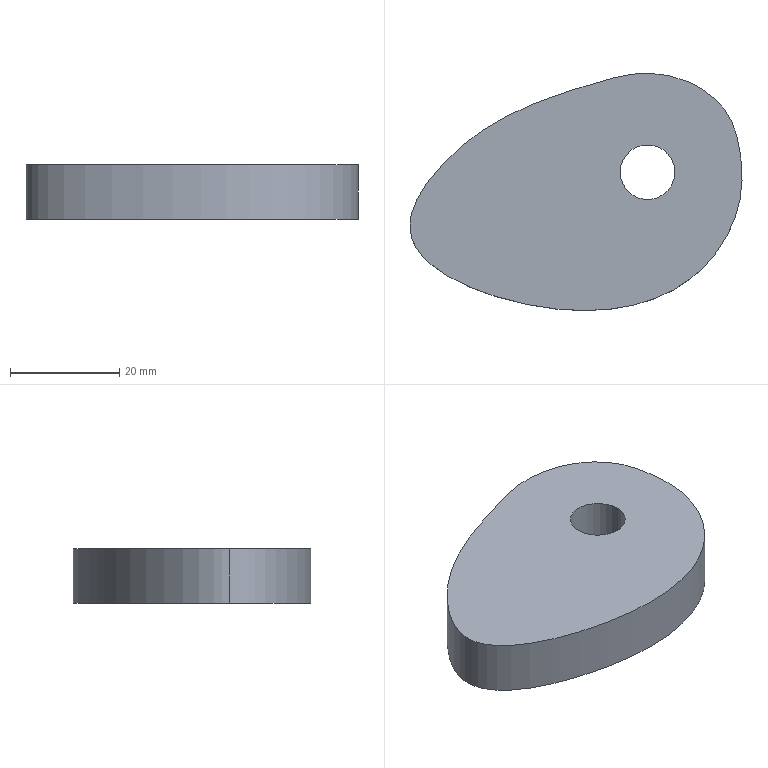Part | SolidWorks | features Extrusion 1 | 1 solid | 6 faces | box 60.725 x 43.378 x 10 mm | volume 18972 mm3 | cylinder 2 | spline 2 | plane 2 | commonest cylinder face diameters 10 x2
STEP:
#1=CARTESIAN_POINT('',(-5.,0.,10.));
#2=VERTEX_POINT('',#1);
#3=CARTESIAN_POINT('',(5.,0.,10.));
#4=VERTEX_POINT('',#3);
#5=CARTESIAN_POINT('',(0.,0.,10.));
#6=DIRECTION('',(0.,0.,1.));
#7=DIRECTION('',(1.,0.,0.));
#8=AXIS2_PLACEMENT_3D('',#5,#6,#7);
#9=CIRCLE('',#8,5.);
#10=EDGE_CURVE('',#2,#4,#9,.T.);
#11=ORIENTED_EDGE('',*,*,#10,.T.);
#12=CARTESIAN_POINT('',(5.,0.,0.));
#13=VERTEX_POINT('',#12);
#14=CARTESIAN_POINT('',(5.,0.,10.));
#15=DIRECTION('',(0.,0.,-1.));
#16=VECTOR('',#15,1000.);
#17=LINE('',#14,#16);
#18=EDGE_CURVE('',#4,#13,#17,.T.);
#19=ORIENTED_EDGE('',*,*,#18,.T.);
#20=CARTESIAN_POINT('',(-5.,0.,0.));
#21=VERTEX_POINT('',#20);
#22=CARTESIAN_POINT('',(0.,0.,0.));
#23=DIRECTION('',(0.,0.,1.));
#24=DIRECTION('',(1.,0.,0.));
#25=AXIS2_PLACEMENT_3D('',#22,#23,#24);
#26=CIRCLE('',#25,5.);
#27=EDGE_CURVE('',#21,#13,#26,.T.);
#28=ORIENTED_EDGE('',*,*,#27,.F.);
#29=CARTESIAN_POINT('',(-5.,0.,10.));
#30=DIRECTION('',(0.,0.,-1.));
#31=VECTOR('',#30,1000.);
#32=LINE('',#29,#31);
#33=EDGE_CURVE('',#2,#21,#32,.T.);
#34=ORIENTED_EDGE('',*,*,#33,.F.);
#35=EDGE_LOOP('',(#11,#19,#28,#34));
#36=FACE_OUTER_BOUND('',#35,.T.);
#37=CARTESIAN_POINT('',(0.,0.,10.));
#38=DIRECTION('',(0.,0.,-1.));
#39=DIRECTION('',(-1.,0.,0.));
#40=AXIS2_PLACEMENT_3D('',#37,#38,#39);
#41=CYLINDRICAL_SURFACE('',#40,5.);
#42=ADVANCED_FACE('',(#36),#41,.F.);
#43=CARTESIAN_POINT('',(-43.419,-10.499,10.));
#44=VERTEX_POINT('',#43);
#45=CARTESIAN_POINT('',(17.013,2.958,10.));
#46=VERTEX_POINT('',#45);
#47=CARTESIAN_POINT('',(-43.419,-10.499,10.));
#48=CARTESIAN_POINT('',(-42.752,-17.454,10.));
#49=CARTESIAN_POINT('',(-17.056,-28.779,10.));
#50=CARTESIAN_POINT('',(9.041,-23.635,10.));
#51=CARTESIAN_POINT('',(17.515,-6.091,10.));
#52=CARTESIAN_POINT('',(17.324,0.4877,10.));
#53=CARTESIAN_POINT('',(17.013,2.958,10.));
#54=B_SPLINE_CURVE_WITH_KNOTS('',3,(#47,#48,#49,#50,#51,#52,#53),.UNSPECIFIED.,.F.,.F.,(4,1,1,1,4),(0.5,0.6591,0.8767,0.9539,1.),.UNSPECIFIED.);
#55=EDGE_CURVE('',#44,#46,#54,.T.);
#56=ORIENTED_EDGE('',*,*,#55,.F.);
#57=CARTESIAN_POINT('',(-43.419,-10.499,0.));
#58=VERTEX_POINT('',#57);
#59=CARTESIAN_POINT('',(-43.419,-10.499,10.));
#60=DIRECTION('',(0.,0.,-1.));
#61=VECTOR('',#60,1000.);
#62=LINE('',#59,#61);
#63=EDGE_CURVE('',#44,#58,#62,.T.);
#64=ORIENTED_EDGE('',*,*,#63,.T.);
#65=CARTESIAN_POINT('',(17.013,2.958,0.));
#66=VERTEX_POINT('',#65);
#67=CARTESIAN_POINT('',(-43.419,-10.499,0.));
#68=CARTESIAN_POINT('',(-42.752,-17.454,0.));
#69=CARTESIAN_POINT('',(-17.056,-28.779,0.));
#70=CARTESIAN_POINT('',(9.041,-23.635,0.));
#71=CARTESIAN_POINT('',(17.515,-6.091,0.));
#72=CARTESIAN_POINT('',(17.324,0.4877,0.));
#73=CARTESIAN_POINT('',(17.013,2.958,0.));
#74=B_SPLINE_CURVE_WITH_KNOTS('',3,(#67,#68,#69,#70,#71,#72,#73),.UNSPECIFIED.,.F.,.F.,(4,1,1,1,4),(0.5,0.6591,0.8767,0.9539,1.),.UNSPECIFIED.);
#75=EDGE_CURVE('',#58,#66,#74,.T.);
#76=ORIENTED_EDGE('',*,*,#75,.T.);
#77=CARTESIAN_POINT('',(17.013,2.958,10.));
#78=DIRECTION('',(0.,0.,-1.));
#79=VECTOR('',#78,1000.);
#80=LINE('',#77,#79);
#81=EDGE_CURVE('',#46,#66,#80,.T.);
#82=ORIENTED_EDGE('',*,*,#81,.F.);
#83=EDGE_LOOP('',(#56,#64,#76,#82));
#84=FACE_OUTER_BOUND('',#83,.T.);
#85=CARTESIAN_POINT('',(-43.419,-10.499,10.));
#86=CARTESIAN_POINT('',(-43.419,-10.499,0.));
#87=CARTESIAN_POINT('',(-42.752,-17.454,10.));
#88=CARTESIAN_POINT('',(-42.752,-17.454,0.));
#89=CARTESIAN_POINT('',(-17.056,-28.779,10.));
#90=CARTESIAN_POINT('',(-17.056,-28.779,0.));
#91=CARTESIAN_POINT('',(9.041,-23.635,10.));
#92=CARTESIAN_POINT('',(9.041,-23.635,0.));
#93=CARTESIAN_POINT('',(17.515,-6.091,10.));
#94=CARTESIAN_POINT('',(17.515,-6.091,0.));
#95=CARTESIAN_POINT('',(17.324,0.4877,10.));
#96=CARTESIAN_POINT('',(17.324,0.4877,0.));
#97=CARTESIAN_POINT('',(17.013,2.958,10.));
#98=CARTESIAN_POINT('',(17.013,2.958,0.));
#99=B_SPLINE_SURFACE_WITH_KNOTS('',3,1,((#85,#86),(#87,#88),(#89,#90),(#91,#92),(#93,#94),(#95,#96),(#97,#98)),.UNSPECIFIED.,.F.,.F.,.F.,(4,1,1,1,4),(2,2),(0.5,0.6591,0.8767,0.9539,1.),(0.,1.),.UNSPECIFIED.);
#100=ADVANCED_FACE('',(#84),#99,.F.);
#101=CARTESIAN_POINT('',(17.013,2.958,10.));
#102=CARTESIAN_POINT('',(16.67,5.672,10.));
#103=CARTESIAN_POINT('',(15.377,11.266,10.));
#104=CARTESIAN_POINT('',(8.,17.178,10.));
#105=CARTESIAN_POINT('',(-1.479,18.809,10.));
#106=CARTESIAN_POINT('',(-16.415,14.213,10.));
#107=CARTESIAN_POINT('',(-32.42,9.014,10.));
#108=CARTESIAN_POINT('',(-43.748,-5.66,10.));
#109=CARTESIAN_POINT('',(-43.432,-10.363,10.));
#110=CARTESIAN_POINT('',(-43.419,-10.499,10.));
#111=B_SPLINE_CURVE_WITH_KNOTS('',3,(#101,#102,#103,#104,#105,#106,#107,#108,#109,#110),.UNSPECIFIED.,.F.,.F.,(4,1,1,1,1,1,1,4),(0.,0.05062,0.1037,0.1669,0.2236,0.393,0.4969,0.5),.UNSPECIFIED.);
#112=EDGE_CURVE('',#46,#44,#111,.T.);
#113=ORIENTED_EDGE('',*,*,#112,.T.);
#114=ORIENTED_EDGE('',*,*,#55,.T.);
#115=EDGE_LOOP('',(#113,#114));
#116=FACE_OUTER_BOUND('',#115,.T.);
#117=ORIENTED_EDGE('',*,*,#10,.F.);
#118=CARTESIAN_POINT('',(0.,0.,10.));
#119=DIRECTION('',(0.,0.,1.));
#120=DIRECTION('',(1.,0.,0.));
#121=AXIS2_PLACEMENT_3D('',#118,#119,#120);
#122=CIRCLE('',#121,5.);
#123=EDGE_CURVE('',#4,#2,#122,.T.);
#124=ORIENTED_EDGE('',*,*,#123,.F.);
#125=EDGE_LOOP('',(#117,#124));
#126=FACE_BOUND('',#125,.T.);
#127=CARTESIAN_POINT('',(-43.419,-10.499,10.));
#128=DIRECTION('',(0.,0.,-1.));
#129=DIRECTION('',(-1.,0.,0.));
#130=AXIS2_PLACEMENT_3D('',#127,#128,#129);
#131=PLANE('',#130);
#132=ADVANCED_FACE('',(#116,#126),#131,.F.);
#133=CARTESIAN_POINT('',(17.013,2.958,0.));
#134=CARTESIAN_POINT('',(16.67,5.672,0.));
#135=CARTESIAN_POINT('',(15.377,11.266,0.));
#136=CARTESIAN_POINT('',(8.,17.178,0.));
#137=CARTESIAN_POINT('',(-1.479,18.809,0.));
#138=CARTESIAN_POINT('',(-16.415,14.213,0.));
#139=CARTESIAN_POINT('',(-32.42,9.014,0.));
#140=CARTESIAN_POINT('',(-43.748,-5.66,0.));
#141=CARTESIAN_POINT('',(-43.432,-10.363,0.));
#142=CARTESIAN_POINT('',(-43.419,-10.499,0.));
#143=B_SPLINE_CURVE_WITH_KNOTS('',3,(#133,#134,#135,#136,#137,#138,#139,#140,#141,#142),.UNSPECIFIED.,.F.,.F.,(4,1,1,1,1,1,1,4),(0.,0.05062,0.1037,0.1669,0.2236,0.393,0.4969,0.5),.UNSPECIFIED.);
#144=EDGE_CURVE('',#66,#58,#143,.T.);
#145=ORIENTED_EDGE('',*,*,#144,.F.);
#146=ORIENTED_EDGE('',*,*,#75,.F.);
#147=EDGE_LOOP('',(#145,#146));
#148=FACE_OUTER_BOUND('',#147,.T.);
#149=ORIENTED_EDGE('',*,*,#27,.T.);
#150=CARTESIAN_POINT('',(0.,0.,0.));
#151=DIRECTION('',(0.,0.,1.));
#152=DIRECTION('',(1.,0.,0.));
#153=AXIS2_PLACEMENT_3D('',#150,#151,#152);
#154=CIRCLE('',#153,5.);
#155=EDGE_CURVE('',#13,#21,#154,.T.);
#156=ORIENTED_EDGE('',*,*,#155,.T.);
#157=EDGE_LOOP('',(#149,#156));
#158=FACE_BOUND('',#157,.T.);
#159=CARTESIAN_POINT('',(-43.419,-10.499,0.));
#160=DIRECTION('',(0.,0.,-1.));
#161=DIRECTION('',(-1.,0.,0.));
#162=AXIS2_PLACEMENT_3D('',#159,#160,#161);
#163=PLANE('',#162);
#164=ADVANCED_FACE('',(#148,#158),#163,.T.);
#165=ORIENTED_EDGE('',*,*,#63,.F.);
#166=ORIENTED_EDGE('',*,*,#112,.F.);
#167=ORIENTED_EDGE('',*,*,#81,.T.);
#168=ORIENTED_EDGE('',*,*,#144,.T.);
#169=EDGE_LOOP('',(#165,#166,#167,#168));
#170=FACE_OUTER_BOUND('',#169,.T.);
#171=CARTESIAN_POINT('',(17.013,2.958,10.));
#172=CARTESIAN_POINT('',(17.013,2.958,0.));
#173=CARTESIAN_POINT('',(16.67,5.672,10.));
#174=CARTESIAN_POINT('',(16.67,5.672,0.));
#175=CARTESIAN_POINT('',(15.377,11.266,10.));
#176=CARTESIAN_POINT('',(15.377,11.266,0.));
#177=CARTESIAN_POINT('',(8.,17.178,10.));
#178=CARTESIAN_POINT('',(8.,17.178,0.));
#179=CARTESIAN_POINT('',(-1.479,18.809,10.));
#180=CARTESIAN_POINT('',(-1.479,18.809,0.));
#181=CARTESIAN_POINT('',(-16.415,14.213,10.));
#182=CARTESIAN_POINT('',(-16.415,14.213,0.));
#183=CARTESIAN_POINT('',(-32.42,9.014,10.));
#184=CARTESIAN_POINT('',(-32.42,9.014,0.));
#185=CARTESIAN_POINT('',(-43.748,-5.66,10.));
#186=CARTESIAN_POINT('',(-43.748,-5.66,0.));
#187=CARTESIAN_POINT('',(-43.432,-10.363,10.));
#188=CARTESIAN_POINT('',(-43.432,-10.363,0.));
#189=CARTESIAN_POINT('',(-43.419,-10.499,10.));
#190=CARTESIAN_POINT('',(-43.419,-10.499,0.));
#191=B_SPLINE_SURFACE_WITH_KNOTS('',3,1,((#171,#172),(#173,#174),(#175,#176),(#177,#178),(#179,#180),(#181,#182),(#183,#184),(#185,#186),(#187,#188),(#189,#190)),.UNSPECIFIED.,.F.,.F.,.F.,(4,1,1,1,1,1,1,4),(2,2),(0.,0.05062,0.1037,0.1669,0.2236,0.393,0.4969,0.5),(0.,1.),.UNSPECIFIED.);
#192=ADVANCED_FACE('',(#170),#191,.F.);
#193=ORIENTED_EDGE('',*,*,#18,.F.);
#194=ORIENTED_EDGE('',*,*,#123,.T.);
#195=ORIENTED_EDGE('',*,*,#33,.T.);
#196=ORIENTED_EDGE('',*,*,#155,.F.);
#197=EDGE_LOOP('',(#193,#194,#195,#196));
#198=FACE_OUTER_BOUND('',#197,.T.);
#199=CARTESIAN_POINT('',(0.,0.,10.));
#200=DIRECTION('',(0.,0.,-1.));
#201=DIRECTION('',(-1.,0.,0.));
#202=AXIS2_PLACEMENT_3D('',#199,#200,#201);
#203=CYLINDRICAL_SURFACE('',#202,5.);
#204=ADVANCED_FACE('',(#198),#203,.F.);
#205=CLOSED_SHELL('',(#42,#100,#132,#164,#192,#204));
#206=MANIFOLD_SOLID_BREP('',#205);
#207=CARTESIAN_POINT('',(0.,0.,0.));
#208=DIRECTION('',(0.,0.,1.));
#209=DIRECTION('',(1.,0.,0.));
#210=AXIS2_PLACEMENT_3D('',#207,#208,#209);
#211=(LENGTH_UNIT()NAMED_UNIT(*)SI_UNIT(.MILLI.,.METRE.));
#212=UNCERTAINTY_MEASURE_WITH_UNIT(LENGTH_MEASURE(0.00001),#211,'','');
#213=(NAMED_UNIT(*)PLANE_ANGLE_UNIT()SI_UNIT($,.RADIAN.));
#214=(NAMED_UNIT(*)SI_UNIT($,.STERADIAN.)SOLID_ANGLE_UNIT());
#215=(GEOMETRIC_REPRESENTATION_CONTEXT(3)GLOBAL_UNCERTAINTY_ASSIGNED_CONTEXT((#212))GLOBAL_UNIT_ASSIGNED_CONTEXT((#211,#213,#214))REPRESENTATION_CONTEXT('',''));
#216=ADVANCED_BREP_SHAPE_REPRESENTATION('',(#206,#210),#215);